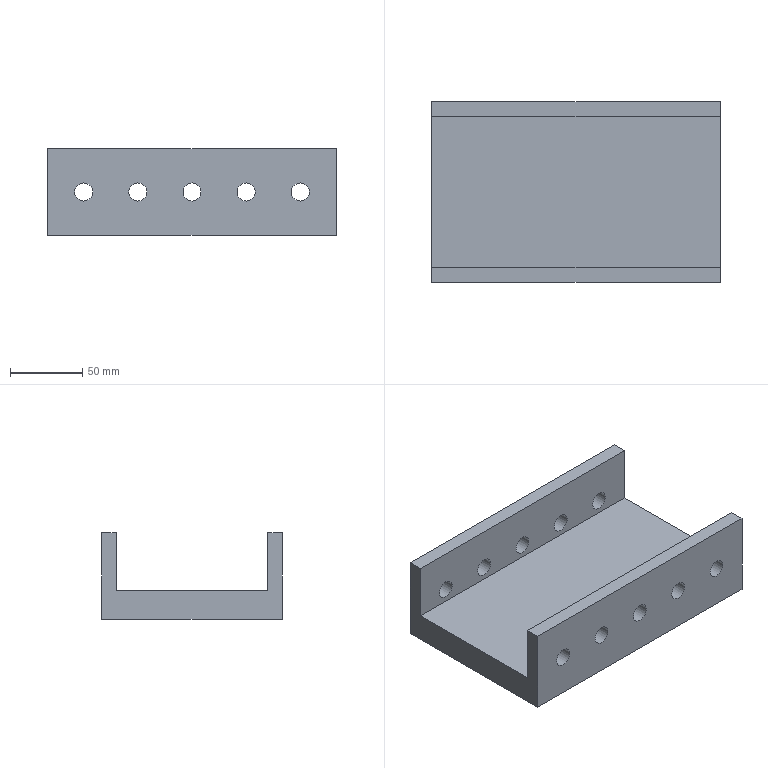Part | NX | features EXTRACT_BODY 5, SIMPLE HOLE 5, DATUM_CSYS 3, EXTRUDE 2, SKETCH 2, CHAMFER 1, Container 1, Geometry Instance 1, HOLE PACKAGE 1, SUBTRACT 1 | 1 solid | 20 faces | box 200 x 125 x 60 mm | volume 647728 mm3 | plane 10 | cylinder 10 | commonest cylinder face diameters 12.5 x10
STEP:
#1=CARTESIAN_POINT('',(175.,115.,23.75));
#2=VERTEX_POINT('',#1);
#3=CARTESIAN_POINT('',(175.,115.,30.));
#4=DIRECTION('',(0.,-1.,0.));
#5=DIRECTION('',(0.,0.,-1.));
#6=AXIS2_PLACEMENT_3D('',#3,#4,#5);
#7=CIRCLE('',#6,6.25);
#8=EDGE_CURVE('',#2,#2,#7,.F.);
#9=ORIENTED_EDGE('',*,*,#8,.T.);
#10=EDGE_LOOP('',(#9));
#11=FACE_BOUND('',#10,.T.);
#12=CARTESIAN_POINT('',(25.,115.,23.75));
#13=VERTEX_POINT('',#12);
#14=CARTESIAN_POINT('',(25.,115.,30.));
#15=DIRECTION('',(0.,-1.,0.));
#16=DIRECTION('',(0.,0.,-1.));
#17=AXIS2_PLACEMENT_3D('',#14,#15,#16);
#18=CIRCLE('',#17,6.25);
#19=EDGE_CURVE('',#13,#13,#18,.F.);
#20=ORIENTED_EDGE('',*,*,#19,.T.);
#21=EDGE_LOOP('',(#20));
#22=FACE_BOUND('',#21,.T.);
#23=CARTESIAN_POINT('',(62.5,115.,23.75));
#24=VERTEX_POINT('',#23);
#25=CARTESIAN_POINT('',(62.5,115.,30.));
#26=DIRECTION('',(0.,-1.,0.));
#27=DIRECTION('',(0.,0.,-1.));
#28=AXIS2_PLACEMENT_3D('',#25,#26,#27);
#29=CIRCLE('',#28,6.25);
#30=EDGE_CURVE('',#24,#24,#29,.F.);
#31=ORIENTED_EDGE('',*,*,#30,.T.);
#32=EDGE_LOOP('',(#31));
#33=FACE_BOUND('',#32,.T.);
#34=CARTESIAN_POINT('',(100.,115.,23.75));
#35=VERTEX_POINT('',#34);
#36=CARTESIAN_POINT('',(100.,115.,30.));
#37=DIRECTION('',(0.,-1.,0.));
#38=DIRECTION('',(0.,0.,-1.));
#39=AXIS2_PLACEMENT_3D('',#36,#37,#38);
#40=CIRCLE('',#39,6.25);
#41=EDGE_CURVE('',#35,#35,#40,.F.);
#42=ORIENTED_EDGE('',*,*,#41,.T.);
#43=EDGE_LOOP('',(#42));
#44=FACE_BOUND('',#43,.T.);
#45=CARTESIAN_POINT('',(137.5,115.,23.75));
#46=VERTEX_POINT('',#45);
#47=CARTESIAN_POINT('',(137.5,115.,30.));
#48=DIRECTION('',(0.,-1.,0.));
#49=DIRECTION('',(0.,0.,-1.));
#50=AXIS2_PLACEMENT_3D('',#47,#48,#49);
#51=CIRCLE('',#50,6.25);
#52=EDGE_CURVE('',#46,#46,#51,.F.);
#53=ORIENTED_EDGE('',*,*,#52,.T.);
#54=EDGE_LOOP('',(#53));
#55=FACE_BOUND('',#54,.T.);
#56=CARTESIAN_POINT('',(200.,115.,20.));
#57=VERTEX_POINT('',#56);
#58=CARTESIAN_POINT('',(0.,115.,20.));
#59=VERTEX_POINT('',#58);
#60=CARTESIAN_POINT('',(200.,115.,20.));
#61=DIRECTION('',(-1.,0.,0.));
#62=VECTOR('',#61,1000.);
#63=LINE('',#60,#62);
#64=EDGE_CURVE('',#57,#59,#63,.T.);
#65=ORIENTED_EDGE('',*,*,#64,.F.);
#66=CARTESIAN_POINT('',(200.,115.,60.));
#67=VERTEX_POINT('',#66);
#68=CARTESIAN_POINT('',(200.,115.,60.));
#69=DIRECTION('',(0.,0.,-1.));
#70=VECTOR('',#69,1000.);
#71=LINE('',#68,#70);
#72=EDGE_CURVE('',#67,#57,#71,.T.);
#73=ORIENTED_EDGE('',*,*,#72,.F.);
#74=CARTESIAN_POINT('',(0.,115.,60.));
#75=VERTEX_POINT('',#74);
#76=CARTESIAN_POINT('',(200.,115.,60.));
#77=DIRECTION('',(-1.,0.,0.));
#78=VECTOR('',#77,1000.);
#79=LINE('',#76,#78);
#80=EDGE_CURVE('',#67,#75,#79,.T.);
#81=ORIENTED_EDGE('',*,*,#80,.T.);
#82=CARTESIAN_POINT('',(0.,115.,60.));
#83=DIRECTION('',(0.,0.,-1.));
#84=VECTOR('',#83,1000.);
#85=LINE('',#82,#84);
#86=EDGE_CURVE('',#75,#59,#85,.T.);
#87=ORIENTED_EDGE('',*,*,#86,.T.);
#88=EDGE_LOOP('',(#65,#73,#81,#87));
#89=FACE_BOUND('',#88,.T.);
#90=CARTESIAN_POINT('',(200.,115.,60.));
#91=DIRECTION('',(0.,1.,0.));
#92=DIRECTION('',(0.,0.,1.));
#93=AXIS2_PLACEMENT_3D('',#90,#91,#92);
#94=PLANE('',#93);
#95=ADVANCED_FACE('',(#11,#22,#33,#44,#55,#89),#94,.F.);
#96=CARTESIAN_POINT('',(175.,10.,23.75));
#97=VERTEX_POINT('',#96);
#98=CARTESIAN_POINT('',(175.,10.,30.));
#99=DIRECTION('',(0.,-1.,0.));
#100=DIRECTION('',(0.,0.,-1.));
#101=AXIS2_PLACEMENT_3D('',#98,#99,#100);
#102=CIRCLE('',#101,6.25);
#103=EDGE_CURVE('',#97,#97,#102,.T.);
#104=ORIENTED_EDGE('',*,*,#103,.T.);
#105=EDGE_LOOP('',(#104));
#106=FACE_BOUND('',#105,.T.);
#107=CARTESIAN_POINT('',(137.5,10.,23.75));
#108=VERTEX_POINT('',#107);
#109=CARTESIAN_POINT('',(137.5,10.,30.));
#110=DIRECTION('',(0.,-1.,0.));
#111=DIRECTION('',(0.,0.,-1.));
#112=AXIS2_PLACEMENT_3D('',#109,#110,#111);
#113=CIRCLE('',#112,6.25);
#114=EDGE_CURVE('',#108,#108,#113,.T.);
#115=ORIENTED_EDGE('',*,*,#114,.T.);
#116=EDGE_LOOP('',(#115));
#117=FACE_BOUND('',#116,.T.);
#118=CARTESIAN_POINT('',(100.,10.,23.75));
#119=VERTEX_POINT('',#118);
#120=CARTESIAN_POINT('',(100.,10.,30.));
#121=DIRECTION('',(0.,-1.,0.));
#122=DIRECTION('',(0.,0.,-1.));
#123=AXIS2_PLACEMENT_3D('',#120,#121,#122);
#124=CIRCLE('',#123,6.25);
#125=EDGE_CURVE('',#119,#119,#124,.T.);
#126=ORIENTED_EDGE('',*,*,#125,.T.);
#127=EDGE_LOOP('',(#126));
#128=FACE_BOUND('',#127,.T.);
#129=CARTESIAN_POINT('',(62.5,10.,23.75));
#130=VERTEX_POINT('',#129);
#131=CARTESIAN_POINT('',(62.5,10.,30.));
#132=DIRECTION('',(0.,-1.,0.));
#133=DIRECTION('',(0.,0.,-1.));
#134=AXIS2_PLACEMENT_3D('',#131,#132,#133);
#135=CIRCLE('',#134,6.25);
#136=EDGE_CURVE('',#130,#130,#135,.T.);
#137=ORIENTED_EDGE('',*,*,#136,.T.);
#138=EDGE_LOOP('',(#137));
#139=FACE_BOUND('',#138,.T.);
#140=CARTESIAN_POINT('',(25.,10.,23.75));
#141=VERTEX_POINT('',#140);
#142=CARTESIAN_POINT('',(25.,10.,30.));
#143=DIRECTION('',(0.,-1.,0.));
#144=DIRECTION('',(0.,0.,-1.));
#145=AXIS2_PLACEMENT_3D('',#142,#143,#144);
#146=CIRCLE('',#145,6.25);
#147=EDGE_CURVE('',#141,#141,#146,.T.);
#148=ORIENTED_EDGE('',*,*,#147,.T.);
#149=EDGE_LOOP('',(#148));
#150=FACE_BOUND('',#149,.T.);
#151=CARTESIAN_POINT('',(0.,10.,20.));
#152=VERTEX_POINT('',#151);
#153=CARTESIAN_POINT('',(200.,10.,20.));
#154=VERTEX_POINT('',#153);
#155=CARTESIAN_POINT('',(0.,10.,20.));
#156=DIRECTION('',(1.,0.,0.));
#157=VECTOR('',#156,1000.);
#158=LINE('',#155,#157);
#159=EDGE_CURVE('',#152,#154,#158,.T.);
#160=ORIENTED_EDGE('',*,*,#159,.F.);
#161=CARTESIAN_POINT('',(0.,10.,60.));
#162=VERTEX_POINT('',#161);
#163=CARTESIAN_POINT('',(0.,10.,10.));
#164=DIRECTION('',(0.,0.,1.));
#165=VECTOR('',#164,1000.);
#166=LINE('',#163,#165);
#167=EDGE_CURVE('',#152,#162,#166,.T.);
#168=ORIENTED_EDGE('',*,*,#167,.T.);
#169=CARTESIAN_POINT('',(200.,10.,60.));
#170=VERTEX_POINT('',#169);
#171=CARTESIAN_POINT('',(200.,10.,60.));
#172=DIRECTION('',(-1.,0.,0.));
#173=VECTOR('',#172,1000.);
#174=LINE('',#171,#173);
#175=EDGE_CURVE('',#170,#162,#174,.T.);
#176=ORIENTED_EDGE('',*,*,#175,.F.);
#177=CARTESIAN_POINT('',(200.,10.,10.));
#178=DIRECTION('',(0.,0.,1.));
#179=VECTOR('',#178,1000.);
#180=LINE('',#177,#179);
#181=EDGE_CURVE('',#154,#170,#180,.T.);
#182=ORIENTED_EDGE('',*,*,#181,.F.);
#183=EDGE_LOOP('',(#160,#168,#176,#182));
#184=FACE_BOUND('',#183,.T.);
#185=CARTESIAN_POINT('',(200.,10.,10.));
#186=DIRECTION('',(0.,-1.,0.));
#187=DIRECTION('',(0.,0.,-1.));
#188=AXIS2_PLACEMENT_3D('',#185,#186,#187);
#189=PLANE('',#188);
#190=ADVANCED_FACE('',(#106,#117,#128,#139,#150,#184),#189,.F.);
#191=CARTESIAN_POINT('',(25.,0.,36.25));
#192=VERTEX_POINT('',#191);
#193=CARTESIAN_POINT('',(25.,0.,30.));
#194=DIRECTION('',(0.,1.,0.));
#195=DIRECTION('',(0.,0.,1.));
#196=AXIS2_PLACEMENT_3D('',#193,#194,#195);
#197=CIRCLE('',#196,6.25);
#198=EDGE_CURVE('',#192,#192,#197,.F.);
#199=ORIENTED_EDGE('',*,*,#198,.F.);
#200=EDGE_LOOP('',(#199));
#201=FACE_BOUND('',#200,.T.);
#202=CARTESIAN_POINT('',(62.5,0.,36.25));
#203=VERTEX_POINT('',#202);
#204=CARTESIAN_POINT('',(62.5,0.,30.));
#205=DIRECTION('',(0.,1.,0.));
#206=DIRECTION('',(0.,0.,1.));
#207=AXIS2_PLACEMENT_3D('',#204,#205,#206);
#208=CIRCLE('',#207,6.25);
#209=EDGE_CURVE('',#203,#203,#208,.F.);
#210=ORIENTED_EDGE('',*,*,#209,.F.);
#211=EDGE_LOOP('',(#210));
#212=FACE_BOUND('',#211,.T.);
#213=CARTESIAN_POINT('',(100.,0.,36.25));
#214=VERTEX_POINT('',#213);
#215=CARTESIAN_POINT('',(100.,0.,30.));
#216=DIRECTION('',(0.,1.,0.));
#217=DIRECTION('',(0.,0.,1.));
#218=AXIS2_PLACEMENT_3D('',#215,#216,#217);
#219=CIRCLE('',#218,6.25);
#220=EDGE_CURVE('',#214,#214,#219,.F.);
#221=ORIENTED_EDGE('',*,*,#220,.F.);
#222=EDGE_LOOP('',(#221));
#223=FACE_BOUND('',#222,.T.);
#224=CARTESIAN_POINT('',(137.5,0.,36.25));
#225=VERTEX_POINT('',#224);
#226=CARTESIAN_POINT('',(137.5,0.,30.));
#227=DIRECTION('',(0.,1.,0.));
#228=DIRECTION('',(0.,0.,1.));
#229=AXIS2_PLACEMENT_3D('',#226,#227,#228);
#230=CIRCLE('',#229,6.25);
#231=EDGE_CURVE('',#225,#225,#230,.F.);
#232=ORIENTED_EDGE('',*,*,#231,.F.);
#233=EDGE_LOOP('',(#232));
#234=FACE_BOUND('',#233,.T.);
#235=CARTESIAN_POINT('',(175.,0.,36.25));
#236=VERTEX_POINT('',#235);
#237=CARTESIAN_POINT('',(175.,0.,30.));
#238=DIRECTION('',(0.,1.,0.));
#239=DIRECTION('',(0.,0.,1.));
#240=AXIS2_PLACEMENT_3D('',#237,#238,#239);
#241=CIRCLE('',#240,6.25);
#242=EDGE_CURVE('',#236,#236,#241,.F.);
#243=ORIENTED_EDGE('',*,*,#242,.F.);
#244=EDGE_LOOP('',(#243));
#245=FACE_BOUND('',#244,.T.);
#246=CARTESIAN_POINT('',(0.,0.,60.));
#247=VERTEX_POINT('',#246);
#248=CARTESIAN_POINT('',(0.,0.,0.));
#249=VERTEX_POINT('',#248);
#250=CARTESIAN_POINT('',(0.,0.,60.));
#251=DIRECTION('',(0.,0.,-1.));
#252=VECTOR('',#251,1000.);
#253=LINE('',#250,#252);
#254=EDGE_CURVE('',#247,#249,#253,.T.);
#255=ORIENTED_EDGE('',*,*,#254,.T.);
#256=CARTESIAN_POINT('',(200.,0.,0.));
#257=VERTEX_POINT('',#256);
#258=CARTESIAN_POINT('',(200.,0.,0.));
#259=DIRECTION('',(-1.,0.,0.));
#260=VECTOR('',#259,1000.);
#261=LINE('',#258,#260);
#262=EDGE_CURVE('',#257,#249,#261,.T.);
#263=ORIENTED_EDGE('',*,*,#262,.F.);
#264=CARTESIAN_POINT('',(200.,0.,60.));
#265=VERTEX_POINT('',#264);
#266=CARTESIAN_POINT('',(200.,0.,60.));
#267=DIRECTION('',(0.,0.,-1.));
#268=VECTOR('',#267,1000.);
#269=LINE('',#266,#268);
#270=EDGE_CURVE('',#265,#257,#269,.T.);
#271=ORIENTED_EDGE('',*,*,#270,.F.);
#272=CARTESIAN_POINT('',(200.,0.,60.));
#273=DIRECTION('',(-1.,0.,0.));
#274=VECTOR('',#273,1000.);
#275=LINE('',#272,#274);
#276=EDGE_CURVE('',#265,#247,#275,.T.);
#277=ORIENTED_EDGE('',*,*,#276,.T.);
#278=EDGE_LOOP('',(#255,#263,#271,#277));
#279=FACE_BOUND('',#278,.T.);
#280=CARTESIAN_POINT('',(200.,0.,60.));
#281=DIRECTION('',(0.,1.,0.));
#282=DIRECTION('',(0.,0.,1.));
#283=AXIS2_PLACEMENT_3D('',#280,#281,#282);
#284=PLANE('',#283);
#285=ADVANCED_FACE('',(#201,#212,#223,#234,#245,#279),#284,.F.);
#286=CARTESIAN_POINT('',(0.,125.,0.));
#287=VERTEX_POINT('',#286);
#288=CARTESIAN_POINT('',(0.,0.,0.));
#289=DIRECTION('',(0.,1.,0.));
#290=VECTOR('',#289,1000.);
#291=LINE('',#288,#290);
#292=EDGE_CURVE('',#249,#287,#291,.T.);
#293=ORIENTED_EDGE('',*,*,#292,.T.);
#294=CARTESIAN_POINT('',(200.,125.,0.));
#295=VERTEX_POINT('',#294);
#296=CARTESIAN_POINT('',(200.,125.,0.));
#297=DIRECTION('',(-1.,0.,0.));
#298=VECTOR('',#297,1000.);
#299=LINE('',#296,#298);
#300=EDGE_CURVE('',#295,#287,#299,.T.);
#301=ORIENTED_EDGE('',*,*,#300,.F.);
#302=CARTESIAN_POINT('',(200.,0.,0.));
#303=DIRECTION('',(0.,1.,0.));
#304=VECTOR('',#303,1000.);
#305=LINE('',#302,#304);
#306=EDGE_CURVE('',#257,#295,#305,.T.);
#307=ORIENTED_EDGE('',*,*,#306,.F.);
#308=ORIENTED_EDGE('',*,*,#262,.T.);
#309=EDGE_LOOP('',(#293,#301,#307,#308));
#310=FACE_BOUND('',#309,.T.);
#311=CARTESIAN_POINT('',(200.,0.,0.));
#312=DIRECTION('',(0.,0.,1.));
#313=DIRECTION('',(0.,-1.,0.));
#314=AXIS2_PLACEMENT_3D('',#311,#312,#313);
#315=PLANE('',#314);
#316=ADVANCED_FACE('',(#310),#315,.F.);
#317=CARTESIAN_POINT('',(137.5,125.,36.25));
#318=VERTEX_POINT('',#317);
#319=CARTESIAN_POINT('',(137.5,125.,30.));
#320=DIRECTION('',(0.,1.,0.));
#321=DIRECTION('',(0.,0.,1.));
#322=AXIS2_PLACEMENT_3D('',#319,#320,#321);
#323=CIRCLE('',#322,6.25);
#324=EDGE_CURVE('',#318,#318,#323,.T.);
#325=ORIENTED_EDGE('',*,*,#324,.F.);
#326=EDGE_LOOP('',(#325));
#327=FACE_BOUND('',#326,.T.);
#328=CARTESIAN_POINT('',(100.,125.,36.25));
#329=VERTEX_POINT('',#328);
#330=CARTESIAN_POINT('',(100.,125.,30.));
#331=DIRECTION('',(0.,1.,0.));
#332=DIRECTION('',(0.,0.,1.));
#333=AXIS2_PLACEMENT_3D('',#330,#331,#332);
#334=CIRCLE('',#333,6.25);
#335=EDGE_CURVE('',#329,#329,#334,.T.);
#336=ORIENTED_EDGE('',*,*,#335,.F.);
#337=EDGE_LOOP('',(#336));
#338=FACE_BOUND('',#337,.T.);
#339=CARTESIAN_POINT('',(62.5,125.,36.25));
#340=VERTEX_POINT('',#339);
#341=CARTESIAN_POINT('',(62.5,125.,30.));
#342=DIRECTION('',(0.,1.,0.));
#343=DIRECTION('',(0.,0.,1.));
#344=AXIS2_PLACEMENT_3D('',#341,#342,#343);
#345=CIRCLE('',#344,6.25);
#346=EDGE_CURVE('',#340,#340,#345,.T.);
#347=ORIENTED_EDGE('',*,*,#346,.F.);
#348=EDGE_LOOP('',(#347));
#349=FACE_BOUND('',#348,.T.);
#350=CARTESIAN_POINT('',(25.,125.,36.25));
#351=VERTEX_POINT('',#350);
#352=CARTESIAN_POINT('',(25.,125.,30.));
#353=DIRECTION('',(0.,1.,0.));
#354=DIRECTION('',(0.,0.,1.));
#355=AXIS2_PLACEMENT_3D('',#352,#353,#354);
#356=CIRCLE('',#355,6.25);
#357=EDGE_CURVE('',#351,#351,#356,.T.);
#358=ORIENTED_EDGE('',*,*,#357,.F.);
#359=EDGE_LOOP('',(#358));
#360=FACE_BOUND('',#359,.T.);
#361=CARTESIAN_POINT('',(175.,125.,36.25));
#362=VERTEX_POINT('',#361);
#363=CARTESIAN_POINT('',(175.,125.,30.));
#364=DIRECTION('',(0.,1.,0.));
#365=DIRECTION('',(0.,0.,1.));
#366=AXIS2_PLACEMENT_3D('',#363,#364,#365);
#367=CIRCLE('',#366,6.25);
#368=EDGE_CURVE('',#362,#362,#367,.T.);
#369=ORIENTED_EDGE('',*,*,#368,.F.);
#370=EDGE_LOOP('',(#369));
#371=FACE_BOUND('',#370,.T.);
#372=CARTESIAN_POINT('',(0.,125.,60.));
#373=VERTEX_POINT('',#372);
#374=CARTESIAN_POINT('',(0.,125.,0.));
#375=DIRECTION('',(0.,0.,1.));
#376=VECTOR('',#375,1000.);
#377=LINE('',#374,#376);
#378=EDGE_CURVE('',#287,#373,#377,.T.);
#379=ORIENTED_EDGE('',*,*,#378,.T.);
#380=CARTESIAN_POINT('',(200.,125.,60.));
#381=VERTEX_POINT('',#380);
#382=CARTESIAN_POINT('',(200.,125.,60.));
#383=DIRECTION('',(-1.,0.,0.));
#384=VECTOR('',#383,1000.);
#385=LINE('',#382,#384);
#386=EDGE_CURVE('',#381,#373,#385,.T.);
#387=ORIENTED_EDGE('',*,*,#386,.F.);
#388=CARTESIAN_POINT('',(200.,125.,0.));
#389=DIRECTION('',(0.,0.,1.));
#390=VECTOR('',#389,1000.);
#391=LINE('',#388,#390);
#392=EDGE_CURVE('',#295,#381,#391,.T.);
#393=ORIENTED_EDGE('',*,*,#392,.F.);
#394=ORIENTED_EDGE('',*,*,#300,.T.);
#395=EDGE_LOOP('',(#379,#387,#393,#394));
#396=FACE_BOUND('',#395,.T.);
#397=CARTESIAN_POINT('',(200.,125.,0.));
#398=DIRECTION('',(0.,-1.,0.));
#399=DIRECTION('',(0.,0.,-1.));
#400=AXIS2_PLACEMENT_3D('',#397,#398,#399);
#401=PLANE('',#400);
#402=ADVANCED_FACE('',(#327,#338,#349,#360,#371,#396),#401,.F.);
#403=CARTESIAN_POINT('',(0.,125.,60.));
#404=DIRECTION('',(0.,-1.,0.));
#405=VECTOR('',#404,1000.);
#406=LINE('',#403,#405);
#407=EDGE_CURVE('',#373,#75,#406,.T.);
#408=ORIENTED_EDGE('',*,*,#407,.T.);
#409=ORIENTED_EDGE('',*,*,#80,.F.);
#410=CARTESIAN_POINT('',(200.,125.,60.));
#411=DIRECTION('',(0.,-1.,0.));
#412=VECTOR('',#411,1000.);
#413=LINE('',#410,#412);
#414=EDGE_CURVE('',#381,#67,#413,.T.);
#415=ORIENTED_EDGE('',*,*,#414,.F.);
#416=ORIENTED_EDGE('',*,*,#386,.T.);
#417=EDGE_LOOP('',(#408,#409,#415,#416));
#418=FACE_BOUND('',#417,.T.);
#419=CARTESIAN_POINT('',(200.,125.,60.));
#420=DIRECTION('',(0.,0.,-1.));
#421=DIRECTION('',(-1.,0.,0.));
#422=AXIS2_PLACEMENT_3D('',#419,#420,#421);
#423=PLANE('',#422);
#424=ADVANCED_FACE('',(#418),#423,.F.);
#425=CARTESIAN_POINT('',(0.,10.,60.));
#426=DIRECTION('',(0.,-1.,0.));
#427=VECTOR('',#426,1000.);
#428=LINE('',#425,#427);
#429=EDGE_CURVE('',#162,#247,#428,.T.);
#430=ORIENTED_EDGE('',*,*,#429,.T.);
#431=ORIENTED_EDGE('',*,*,#276,.F.);
#432=CARTESIAN_POINT('',(200.,10.,60.));
#433=DIRECTION('',(0.,-1.,0.));
#434=VECTOR('',#433,1000.);
#435=LINE('',#432,#434);
#436=EDGE_CURVE('',#170,#265,#435,.T.);
#437=ORIENTED_EDGE('',*,*,#436,.F.);
#438=ORIENTED_EDGE('',*,*,#175,.T.);
#439=EDGE_LOOP('',(#430,#431,#437,#438));
#440=FACE_BOUND('',#439,.T.);
#441=CARTESIAN_POINT('',(200.,10.,60.));
#442=DIRECTION('',(0.,0.,-1.));
#443=DIRECTION('',(-1.,0.,0.));
#444=AXIS2_PLACEMENT_3D('',#441,#442,#443);
#445=PLANE('',#444);
#446=ADVANCED_FACE('',(#440),#445,.F.);
#447=ORIENTED_EDGE('',*,*,#270,.T.);
#448=ORIENTED_EDGE('',*,*,#306,.T.);
#449=ORIENTED_EDGE('',*,*,#392,.T.);
#450=ORIENTED_EDGE('',*,*,#414,.T.);
#451=ORIENTED_EDGE('',*,*,#72,.T.);
#452=CARTESIAN_POINT('',(200.,10.,20.));
#453=DIRECTION('',(0.,1.,0.));
#454=VECTOR('',#453,1000.);
#455=LINE('',#452,#454);
#456=EDGE_CURVE('',#154,#57,#455,.T.);
#457=ORIENTED_EDGE('',*,*,#456,.F.);
#458=ORIENTED_EDGE('',*,*,#181,.T.);
#459=ORIENTED_EDGE('',*,*,#436,.T.);
#460=EDGE_LOOP('',(#447,#448,#449,#450,#451,#457,#458,#459));
#461=FACE_BOUND('',#460,.T.);
#462=CARTESIAN_POINT('',(200.,0.,0.));
#463=DIRECTION('',(1.,0.,0.));
#464=DIRECTION('',(0.,0.,-1.));
#465=AXIS2_PLACEMENT_3D('',#462,#463,#464);
#466=PLANE('',#465);
#467=ADVANCED_FACE('',(#461),#466,.T.);
#468=ORIENTED_EDGE('',*,*,#254,.F.);
#469=ORIENTED_EDGE('',*,*,#429,.F.);
#470=ORIENTED_EDGE('',*,*,#167,.F.);
#471=CARTESIAN_POINT('',(0.,115.,20.));
#472=DIRECTION('',(0.,-1.,0.));
#473=VECTOR('',#472,1000.);
#474=LINE('',#471,#473);
#475=EDGE_CURVE('',#59,#152,#474,.T.);
#476=ORIENTED_EDGE('',*,*,#475,.F.);
#477=ORIENTED_EDGE('',*,*,#86,.F.);
#478=ORIENTED_EDGE('',*,*,#407,.F.);
#479=ORIENTED_EDGE('',*,*,#378,.F.);
#480=ORIENTED_EDGE('',*,*,#292,.F.);
#481=EDGE_LOOP('',(#468,#469,#470,#476,#477,#478,#479,#480));
#482=FACE_BOUND('',#481,.T.);
#483=CARTESIAN_POINT('',(0.,0.,0.));
#484=DIRECTION('',(1.,0.,0.));
#485=DIRECTION('',(0.,0.,-1.));
#486=AXIS2_PLACEMENT_3D('',#483,#484,#485);
#487=PLANE('',#486);
#488=ADVANCED_FACE('',(#482),#487,.F.);
#489=ORIENTED_EDGE('',*,*,#242,.T.);
#490=EDGE_LOOP('',(#489));
#491=FACE_BOUND('',#490,.T.);
#492=ORIENTED_EDGE('',*,*,#103,.F.);
#493=EDGE_LOOP('',(#492));
#494=FACE_BOUND('',#493,.T.);
#495=CARTESIAN_POINT('',(175.,10.,30.));
#496=DIRECTION('',(0.,-1.,0.));
#497=DIRECTION('',(0.,0.,-1.));
#498=AXIS2_PLACEMENT_3D('',#495,#496,#497);
#499=CYLINDRICAL_SURFACE('',#498,6.25);
#500=ADVANCED_FACE('',(#491,#494),#499,.F.);
#501=ORIENTED_EDGE('',*,*,#231,.T.);
#502=EDGE_LOOP('',(#501));
#503=FACE_BOUND('',#502,.T.);
#504=ORIENTED_EDGE('',*,*,#114,.F.);
#505=EDGE_LOOP('',(#504));
#506=FACE_BOUND('',#505,.T.);
#507=CARTESIAN_POINT('',(137.5,10.,30.));
#508=DIRECTION('',(0.,-1.,0.));
#509=DIRECTION('',(0.,0.,-1.));
#510=AXIS2_PLACEMENT_3D('',#507,#508,#509);
#511=CYLINDRICAL_SURFACE('',#510,6.25);
#512=ADVANCED_FACE('',(#503,#506),#511,.F.);
#513=ORIENTED_EDGE('',*,*,#220,.T.);
#514=EDGE_LOOP('',(#513));
#515=FACE_BOUND('',#514,.T.);
#516=ORIENTED_EDGE('',*,*,#125,.F.);
#517=EDGE_LOOP('',(#516));
#518=FACE_BOUND('',#517,.T.);
#519=CARTESIAN_POINT('',(100.,10.,30.));
#520=DIRECTION('',(0.,-1.,0.));
#521=DIRECTION('',(0.,0.,-1.));
#522=AXIS2_PLACEMENT_3D('',#519,#520,#521);
#523=CYLINDRICAL_SURFACE('',#522,6.25);
#524=ADVANCED_FACE('',(#515,#518),#523,.F.);
#525=ORIENTED_EDGE('',*,*,#209,.T.);
#526=EDGE_LOOP('',(#525));
#527=FACE_BOUND('',#526,.T.);
#528=ORIENTED_EDGE('',*,*,#136,.F.);
#529=EDGE_LOOP('',(#528));
#530=FACE_BOUND('',#529,.T.);
#531=CARTESIAN_POINT('',(62.5,10.,30.));
#532=DIRECTION('',(0.,-1.,0.));
#533=DIRECTION('',(0.,0.,-1.));
#534=AXIS2_PLACEMENT_3D('',#531,#532,#533);
#535=CYLINDRICAL_SURFACE('',#534,6.25);
#536=ADVANCED_FACE('',(#527,#530),#535,.F.);
#537=ORIENTED_EDGE('',*,*,#198,.T.);
#538=EDGE_LOOP('',(#537));
#539=FACE_BOUND('',#538,.T.);
#540=ORIENTED_EDGE('',*,*,#147,.F.);
#541=EDGE_LOOP('',(#540));
#542=FACE_BOUND('',#541,.T.);
#543=CARTESIAN_POINT('',(25.,10.,30.));
#544=DIRECTION('',(0.,-1.,0.));
#545=DIRECTION('',(0.,0.,-1.));
#546=AXIS2_PLACEMENT_3D('',#543,#544,#545);
#547=CYLINDRICAL_SURFACE('',#546,6.25);
#548=ADVANCED_FACE('',(#539,#542),#547,.F.);
#549=ORIENTED_EDGE('',*,*,#368,.T.);
#550=EDGE_LOOP('',(#549));
#551=FACE_BOUND('',#550,.T.);
#552=ORIENTED_EDGE('',*,*,#8,.F.);
#553=EDGE_LOOP('',(#552));
#554=FACE_BOUND('',#553,.T.);
#555=CARTESIAN_POINT('',(175.,115.,30.));
#556=DIRECTION('',(0.,1.,0.));
#557=DIRECTION('',(0.,0.,-1.));
#558=AXIS2_PLACEMENT_3D('',#555,#556,#557);
#559=CYLINDRICAL_SURFACE('',#558,6.25);
#560=ADVANCED_FACE('',(#551,#554),#559,.F.);
#561=ORIENTED_EDGE('',*,*,#357,.T.);
#562=EDGE_LOOP('',(#561));
#563=FACE_BOUND('',#562,.T.);
#564=ORIENTED_EDGE('',*,*,#19,.F.);
#565=EDGE_LOOP('',(#564));
#566=FACE_BOUND('',#565,.T.);
#567=CARTESIAN_POINT('',(25.,115.,30.));
#568=DIRECTION('',(0.,1.,0.));
#569=DIRECTION('',(0.,0.,-1.));
#570=AXIS2_PLACEMENT_3D('',#567,#568,#569);
#571=CYLINDRICAL_SURFACE('',#570,6.25);
#572=ADVANCED_FACE('',(#563,#566),#571,.F.);
#573=ORIENTED_EDGE('',*,*,#346,.T.);
#574=EDGE_LOOP('',(#573));
#575=FACE_BOUND('',#574,.T.);
#576=ORIENTED_EDGE('',*,*,#30,.F.);
#577=EDGE_LOOP('',(#576));
#578=FACE_BOUND('',#577,.T.);
#579=CARTESIAN_POINT('',(62.5,115.,30.));
#580=DIRECTION('',(0.,1.,0.));
#581=DIRECTION('',(0.,0.,-1.));
#582=AXIS2_PLACEMENT_3D('',#579,#580,#581);
#583=CYLINDRICAL_SURFACE('',#582,6.25);
#584=ADVANCED_FACE('',(#575,#578),#583,.F.);
#585=ORIENTED_EDGE('',*,*,#335,.T.);
#586=EDGE_LOOP('',(#585));
#587=FACE_BOUND('',#586,.T.);
#588=ORIENTED_EDGE('',*,*,#41,.F.);
#589=EDGE_LOOP('',(#588));
#590=FACE_BOUND('',#589,.T.);
#591=CARTESIAN_POINT('',(100.,115.,30.));
#592=DIRECTION('',(0.,1.,0.));
#593=DIRECTION('',(0.,0.,-1.));
#594=AXIS2_PLACEMENT_3D('',#591,#592,#593);
#595=CYLINDRICAL_SURFACE('',#594,6.25);
#596=ADVANCED_FACE('',(#587,#590),#595,.F.);
#597=ORIENTED_EDGE('',*,*,#324,.T.);
#598=EDGE_LOOP('',(#597));
#599=FACE_BOUND('',#598,.T.);
#600=ORIENTED_EDGE('',*,*,#52,.F.);
#601=EDGE_LOOP('',(#600));
#602=FACE_BOUND('',#601,.T.);
#603=CARTESIAN_POINT('',(137.5,115.,30.));
#604=DIRECTION('',(0.,1.,0.));
#605=DIRECTION('',(0.,0.,-1.));
#606=AXIS2_PLACEMENT_3D('',#603,#604,#605);
#607=CYLINDRICAL_SURFACE('',#606,6.25);
#608=ADVANCED_FACE('',(#599,#602),#607,.F.);
#609=ORIENTED_EDGE('',*,*,#475,.T.);
#610=ORIENTED_EDGE('',*,*,#159,.T.);
#611=ORIENTED_EDGE('',*,*,#456,.T.);
#612=ORIENTED_EDGE('',*,*,#64,.T.);
#613=EDGE_LOOP('',(#609,#610,#611,#612));
#614=FACE_BOUND('',#613,.T.);
#615=CARTESIAN_POINT('',(0.,0.,20.));
#616=DIRECTION('',(0.,0.,1.));
#617=DIRECTION('',(1.,0.,0.));
#618=AXIS2_PLACEMENT_3D('',#615,#616,#617);
#619=PLANE('',#618);
#620=ADVANCED_FACE('',(#614),#619,.T.);
#621=CLOSED_SHELL('',(#95,#190,#285,#316,#402,#424,#446,#467,#488,#500,#512,#524,#536,#548,#560,#572,#584,#596,#608,#620));
#622=MANIFOLD_SOLID_BREP('',#621);
#623=(LENGTH_UNIT()NAMED_UNIT(*)SI_UNIT(.MILLI.,.METRE.));
#624=UNCERTAINTY_MEASURE_WITH_UNIT(LENGTH_MEASURE(0.00001),#623,'','');
#625=(NAMED_UNIT(*)PLANE_ANGLE_UNIT()SI_UNIT($,.RADIAN.));
#626=(NAMED_UNIT(*)SI_UNIT($,.STERADIAN.)SOLID_ANGLE_UNIT());
#627=(GEOMETRIC_REPRESENTATION_CONTEXT(3)GLOBAL_UNCERTAINTY_ASSIGNED_CONTEXT((#624))GLOBAL_UNIT_ASSIGNED_CONTEXT((#623,#625,#626))REPRESENTATION_CONTEXT('',''));
#628=ADVANCED_BREP_SHAPE_REPRESENTATION('',(#622),#627);